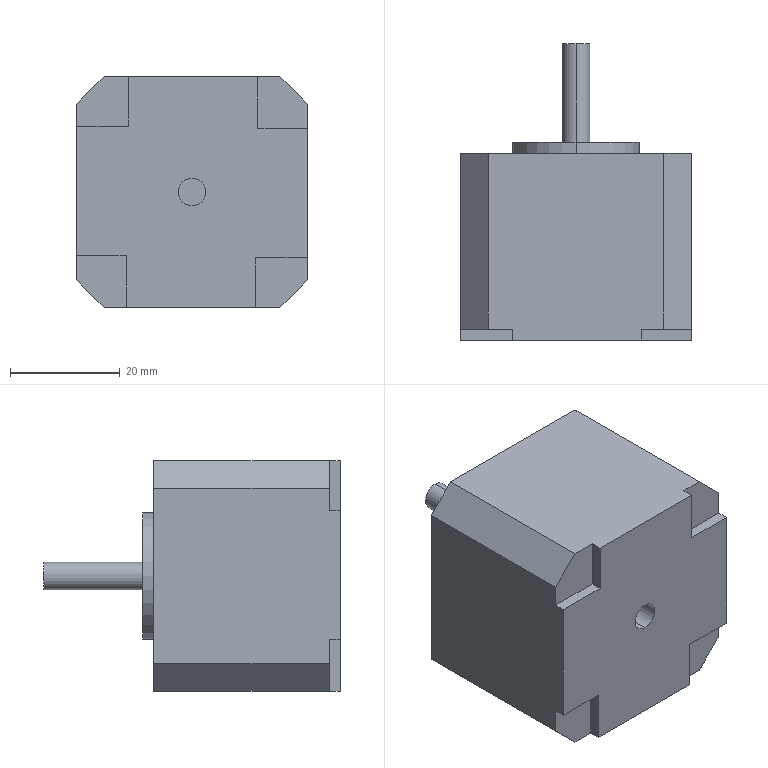Part | STEP file | 42 stepper motor 34 | 1 solid | 49 faces | box 42 x 54 x 42 mm | volume 57864 mm3 | plane 31 | cylinder 18 | commonest cylinder face diameters 3 x8 5 x4 19.644 x2 23 x2 28 x2